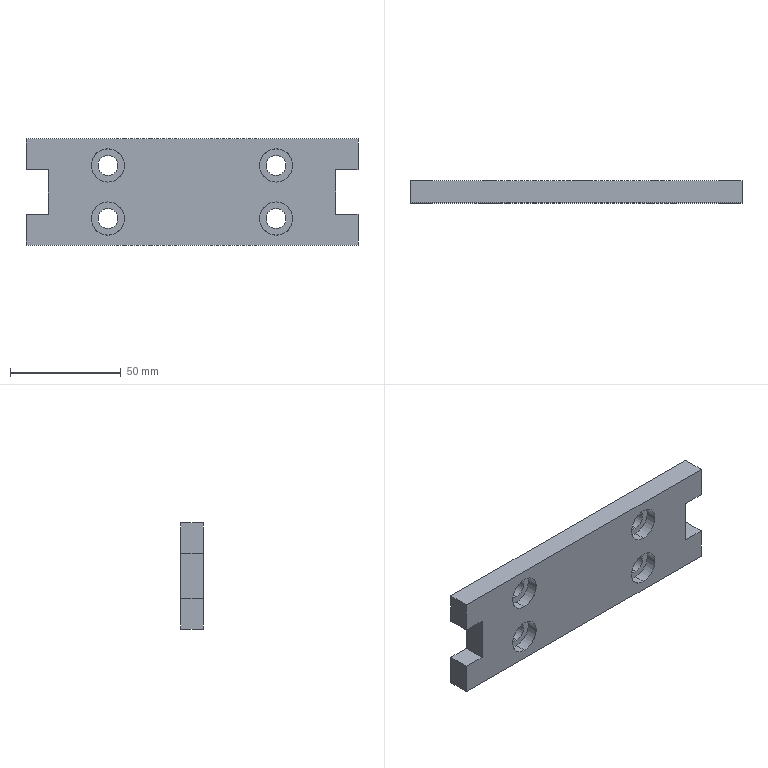Part | SolidWorks | features ICE 2, Extrusion 1, HoleWzd 1 | 1 solid | 45 faces | box 150 x 10 x 48 mm | volume 62310 mm3 | plane 19 | cylinder 18 | cone 8 | commonest cylinder face diameters 15 x10 9 x8
STEP:
#1=CARTESIAN_POINT('',(0.,5.,-7.5));
#2=VERTEX_POINT('',#1);
#3=CARTESIAN_POINT('',(0.,5.,7.5));
#4=VERTEX_POINT('',#3);
#5=CARTESIAN_POINT('',(0.,5.,0.));
#6=DIRECTION('',(0.,1.,0.));
#7=DIRECTION('',(0.,0.,1.));
#8=AXIS2_PLACEMENT_3D('',#5,#6,#7);
#9=CIRCLE('',#8,7.5);
#10=EDGE_CURVE('',#2,#4,#9,.T.);
#11=ORIENTED_EDGE('',*,*,#10,.F.);
#12=CARTESIAN_POINT('',(0.,10.,-7.5));
#13=VERTEX_POINT('',#12);
#14=CARTESIAN_POINT('',(0.,5.,-7.5));
#15=DIRECTION('',(0.,1.,0.));
#16=VECTOR('',#15,1000.);
#17=LINE('',#14,#16);
#18=EDGE_CURVE('',#2,#13,#17,.T.);
#19=ORIENTED_EDGE('',*,*,#18,.T.);
#20=CARTESIAN_POINT('',(0.,10.,7.5));
#21=VERTEX_POINT('',#20);
#22=CARTESIAN_POINT('',(0.,10.,0.));
#23=DIRECTION('',(0.,1.,0.));
#24=DIRECTION('',(0.,0.,1.));
#25=AXIS2_PLACEMENT_3D('',#22,#23,#24);
#26=CIRCLE('',#25,7.5);
#27=EDGE_CURVE('',#13,#21,#26,.T.);
#28=ORIENTED_EDGE('',*,*,#27,.T.);
#29=CARTESIAN_POINT('',(0.,5.,7.5));
#30=DIRECTION('',(0.,1.,0.));
#31=VECTOR('',#30,1000.);
#32=LINE('',#29,#31);
#33=EDGE_CURVE('',#4,#21,#32,.T.);
#34=ORIENTED_EDGE('',*,*,#33,.F.);
#35=EDGE_LOOP('',(#11,#19,#28,#34));
#36=FACE_OUTER_BOUND('',#35,.T.);
#37=CARTESIAN_POINT('',(0.,5.,0.));
#38=DIRECTION('',(0.,1.,0.));
#39=DIRECTION('',(0.,0.,1.));
#40=AXIS2_PLACEMENT_3D('',#37,#38,#39);
#41=CYLINDRICAL_SURFACE('',#40,7.5);
#42=ADVANCED_FACE('',(#36),#41,.F.);
#43=CARTESIAN_POINT('',(38.,0.025,19.5));
#44=VERTEX_POINT('',#43);
#45=CARTESIAN_POINT('',(38.,0.025,4.5));
#46=VERTEX_POINT('',#45);
#47=CARTESIAN_POINT('',(38.,0.025,12.));
#48=DIRECTION('',(0.,-1.,0.));
#49=DIRECTION('',(0.,0.,-1.));
#50=AXIS2_PLACEMENT_3D('',#47,#48,#49);
#51=CIRCLE('',#50,7.5);
#52=EDGE_CURVE('',#44,#46,#51,.T.);
#53=ORIENTED_EDGE('',*,*,#52,.F.);
#54=CARTESIAN_POINT('',(38.,0.,19.525));
#55=VERTEX_POINT('',#54);
#56=CARTESIAN_POINT('',(38.,0.,19.525));
#57=DIRECTION('',(0.,-0.7071,0.7071));
#58=VECTOR('',#57,1000.);
#59=LINE('',#56,#58);
#60=EDGE_CURVE('',#44,#55,#59,.T.);
#61=ORIENTED_EDGE('',*,*,#60,.T.);
#62=CARTESIAN_POINT('',(38.,0.,4.475));
#63=VERTEX_POINT('',#62);
#64=CARTESIAN_POINT('',(38.,0.,12.));
#65=DIRECTION('',(0.,-1.,0.));
#66=DIRECTION('',(0.,0.,-1.));
#67=AXIS2_PLACEMENT_3D('',#64,#65,#66);
#68=CIRCLE('',#67,7.525);
#69=EDGE_CURVE('',#55,#63,#68,.T.);
#70=ORIENTED_EDGE('',*,*,#69,.T.);
#71=CARTESIAN_POINT('',(38.,0.,4.475));
#72=DIRECTION('',(0.,-0.7071,-0.7071));
#73=VECTOR('',#72,1000.);
#74=LINE('',#71,#73);
#75=EDGE_CURVE('',#46,#63,#74,.T.);
#76=ORIENTED_EDGE('',*,*,#75,.F.);
#77=EDGE_LOOP('',(#53,#61,#70,#76));
#78=FACE_OUTER_BOUND('',#77,.T.);
#79=CARTESIAN_POINT('',(38.,0.,12.));
#80=DIRECTION('',(0.,-1.,0.));
#81=DIRECTION('',(0.,0.,-1.));
#82=AXIS2_PLACEMENT_3D('',#79,#80,#81);
#83=CONICAL_SURFACE('',#82,7.525,0.7854);
#84=ADVANCED_FACE('',(#78),#83,.F.);
#85=CARTESIAN_POINT('',(38.,5.,19.5));
#86=VERTEX_POINT('',#85);
#87=CARTESIAN_POINT('',(38.,5.,4.5));
#88=VERTEX_POINT('',#87);
#89=CARTESIAN_POINT('',(38.,5.,12.));
#90=DIRECTION('',(0.,-1.,0.));
#91=DIRECTION('',(0.,0.,-1.));
#92=AXIS2_PLACEMENT_3D('',#89,#90,#91);
#93=CIRCLE('',#92,7.5);
#94=EDGE_CURVE('',#86,#88,#93,.T.);
#95=ORIENTED_EDGE('',*,*,#94,.F.);
#96=CARTESIAN_POINT('',(38.,0.,19.5));
#97=DIRECTION('',(0.,-1.,0.));
#98=VECTOR('',#97,1000.);
#99=LINE('',#96,#98);
#100=EDGE_CURVE('',#86,#44,#99,.T.);
#101=ORIENTED_EDGE('',*,*,#100,.T.);
#102=ORIENTED_EDGE('',*,*,#52,.T.);
#103=CARTESIAN_POINT('',(38.,0.,4.5));
#104=DIRECTION('',(0.,-1.,0.));
#105=VECTOR('',#104,1000.);
#106=LINE('',#103,#105);
#107=EDGE_CURVE('',#88,#46,#106,.T.);
#108=ORIENTED_EDGE('',*,*,#107,.F.);
#109=EDGE_LOOP('',(#95,#101,#102,#108));
#110=FACE_OUTER_BOUND('',#109,.T.);
#111=CARTESIAN_POINT('',(38.,0.,12.));
#112=DIRECTION('',(0.,-1.,0.));
#113=DIRECTION('',(0.,0.,-1.));
#114=AXIS2_PLACEMENT_3D('',#111,#112,#113);
#115=CYLINDRICAL_SURFACE('',#114,7.5);
#116=ADVANCED_FACE('',(#110),#115,.F.);
#117=CARTESIAN_POINT('',(38.,10.,16.5));
#118=VERTEX_POINT('',#117);
#119=CARTESIAN_POINT('',(38.,10.,7.5));
#120=VERTEX_POINT('',#119);
#121=CARTESIAN_POINT('',(38.,10.,12.));
#122=DIRECTION('',(0.,-1.,0.));
#123=DIRECTION('',(0.,0.,-1.));
#124=AXIS2_PLACEMENT_3D('',#121,#122,#123);
#125=CIRCLE('',#124,4.5);
#126=EDGE_CURVE('',#118,#120,#125,.T.);
#127=ORIENTED_EDGE('',*,*,#126,.F.);
#128=CARTESIAN_POINT('',(38.,5.,16.5));
#129=VERTEX_POINT('',#128);
#130=CARTESIAN_POINT('',(38.,0.,16.5));
#131=DIRECTION('',(0.,-1.,0.));
#132=VECTOR('',#131,1000.);
#133=LINE('',#130,#132);
#134=EDGE_CURVE('',#118,#129,#133,.T.);
#135=ORIENTED_EDGE('',*,*,#134,.T.);
#136=CARTESIAN_POINT('',(38.,5.,7.5));
#137=VERTEX_POINT('',#136);
#138=CARTESIAN_POINT('',(38.,5.,12.));
#139=DIRECTION('',(0.,-1.,0.));
#140=DIRECTION('',(0.,0.,-1.));
#141=AXIS2_PLACEMENT_3D('',#138,#139,#140);
#142=CIRCLE('',#141,4.5);
#143=EDGE_CURVE('',#129,#137,#142,.T.);
#144=ORIENTED_EDGE('',*,*,#143,.T.);
#145=CARTESIAN_POINT('',(38.,0.,7.5));
#146=DIRECTION('',(0.,-1.,0.));
#147=VECTOR('',#146,1000.);
#148=LINE('',#145,#147);
#149=EDGE_CURVE('',#120,#137,#148,.T.);
#150=ORIENTED_EDGE('',*,*,#149,.F.);
#151=EDGE_LOOP('',(#127,#135,#144,#150));
#152=FACE_OUTER_BOUND('',#151,.T.);
#153=CARTESIAN_POINT('',(38.,0.,12.));
#154=DIRECTION('',(0.,-1.,0.));
#155=DIRECTION('',(0.,0.,-1.));
#156=AXIS2_PLACEMENT_3D('',#153,#154,#155);
#157=CYLINDRICAL_SURFACE('',#156,4.5);
#158=ADVANCED_FACE('',(#152),#157,.F.);
#159=CARTESIAN_POINT('',(-38.,0.025,19.5));
#160=VERTEX_POINT('',#159);
#161=CARTESIAN_POINT('',(-38.,0.025,4.5));
#162=VERTEX_POINT('',#161);
#163=CARTESIAN_POINT('',(-38.,0.025,12.));
#164=DIRECTION('',(0.,-1.,0.));
#165=DIRECTION('',(0.,0.,-1.));
#166=AXIS2_PLACEMENT_3D('',#163,#164,#165);
#167=CIRCLE('',#166,7.5);
#168=EDGE_CURVE('',#160,#162,#167,.T.);
#169=ORIENTED_EDGE('',*,*,#168,.F.);
#170=CARTESIAN_POINT('',(-38.,0.,19.525));
#171=VERTEX_POINT('',#170);
#172=CARTESIAN_POINT('',(-38.,0.,19.525));
#173=DIRECTION('',(0.,-0.7071,0.7071));
#174=VECTOR('',#173,1000.);
#175=LINE('',#172,#174);
#176=EDGE_CURVE('',#160,#171,#175,.T.);
#177=ORIENTED_EDGE('',*,*,#176,.T.);
#178=CARTESIAN_POINT('',(-38.,0.,4.475));
#179=VERTEX_POINT('',#178);
#180=CARTESIAN_POINT('',(-38.,0.,12.));
#181=DIRECTION('',(0.,-1.,0.));
#182=DIRECTION('',(0.,0.,-1.));
#183=AXIS2_PLACEMENT_3D('',#180,#181,#182);
#184=CIRCLE('',#183,7.525);
#185=EDGE_CURVE('',#171,#179,#184,.T.);
#186=ORIENTED_EDGE('',*,*,#185,.T.);
#187=CARTESIAN_POINT('',(-38.,0.,4.475));
#188=DIRECTION('',(0.,-0.7071,-0.7071));
#189=VECTOR('',#188,1000.);
#190=LINE('',#187,#189);
#191=EDGE_CURVE('',#162,#179,#190,.T.);
#192=ORIENTED_EDGE('',*,*,#191,.F.);
#193=EDGE_LOOP('',(#169,#177,#186,#192));
#194=FACE_OUTER_BOUND('',#193,.T.);
#195=CARTESIAN_POINT('',(-38.,0.,12.));
#196=DIRECTION('',(0.,-1.,0.));
#197=DIRECTION('',(0.,0.,-1.));
#198=AXIS2_PLACEMENT_3D('',#195,#196,#197);
#199=CONICAL_SURFACE('',#198,7.525,0.7854);
#200=ADVANCED_FACE('',(#194),#199,.F.);
#201=CARTESIAN_POINT('',(-38.,5.,19.5));
#202=VERTEX_POINT('',#201);
#203=CARTESIAN_POINT('',(-38.,5.,4.5));
#204=VERTEX_POINT('',#203);
#205=CARTESIAN_POINT('',(-38.,5.,12.));
#206=DIRECTION('',(0.,-1.,0.));
#207=DIRECTION('',(0.,0.,-1.));
#208=AXIS2_PLACEMENT_3D('',#205,#206,#207);
#209=CIRCLE('',#208,7.5);
#210=EDGE_CURVE('',#202,#204,#209,.T.);
#211=ORIENTED_EDGE('',*,*,#210,.F.);
#212=CARTESIAN_POINT('',(-38.,0.,19.5));
#213=DIRECTION('',(0.,-1.,0.));
#214=VECTOR('',#213,1000.);
#215=LINE('',#212,#214);
#216=EDGE_CURVE('',#202,#160,#215,.T.);
#217=ORIENTED_EDGE('',*,*,#216,.T.);
#218=ORIENTED_EDGE('',*,*,#168,.T.);
#219=CARTESIAN_POINT('',(-38.,0.,4.5));
#220=DIRECTION('',(0.,-1.,0.));
#221=VECTOR('',#220,1000.);
#222=LINE('',#219,#221);
#223=EDGE_CURVE('',#204,#162,#222,.T.);
#224=ORIENTED_EDGE('',*,*,#223,.F.);
#225=EDGE_LOOP('',(#211,#217,#218,#224));
#226=FACE_OUTER_BOUND('',#225,.T.);
#227=CARTESIAN_POINT('',(-38.,0.,12.));
#228=DIRECTION('',(0.,-1.,0.));
#229=DIRECTION('',(0.,0.,-1.));
#230=AXIS2_PLACEMENT_3D('',#227,#228,#229);
#231=CYLINDRICAL_SURFACE('',#230,7.5);
#232=ADVANCED_FACE('',(#226),#231,.F.);
#233=CARTESIAN_POINT('',(-38.,10.,16.5));
#234=VERTEX_POINT('',#233);
#235=CARTESIAN_POINT('',(-38.,10.,7.5));
#236=VERTEX_POINT('',#235);
#237=CARTESIAN_POINT('',(-38.,10.,12.));
#238=DIRECTION('',(0.,-1.,0.));
#239=DIRECTION('',(0.,0.,-1.));
#240=AXIS2_PLACEMENT_3D('',#237,#238,#239);
#241=CIRCLE('',#240,4.5);
#242=EDGE_CURVE('',#234,#236,#241,.T.);
#243=ORIENTED_EDGE('',*,*,#242,.F.);
#244=CARTESIAN_POINT('',(-38.,5.,16.5));
#245=VERTEX_POINT('',#244);
#246=CARTESIAN_POINT('',(-38.,0.,16.5));
#247=DIRECTION('',(0.,-1.,0.));
#248=VECTOR('',#247,1000.);
#249=LINE('',#246,#248);
#250=EDGE_CURVE('',#234,#245,#249,.T.);
#251=ORIENTED_EDGE('',*,*,#250,.T.);
#252=CARTESIAN_POINT('',(-38.,5.,7.5));
#253=VERTEX_POINT('',#252);
#254=CARTESIAN_POINT('',(-38.,5.,12.));
#255=DIRECTION('',(0.,-1.,0.));
#256=DIRECTION('',(0.,0.,-1.));
#257=AXIS2_PLACEMENT_3D('',#254,#255,#256);
#258=CIRCLE('',#257,4.5);
#259=EDGE_CURVE('',#245,#253,#258,.T.);
#260=ORIENTED_EDGE('',*,*,#259,.T.);
#261=CARTESIAN_POINT('',(-38.,0.,7.5));
#262=DIRECTION('',(0.,-1.,0.));
#263=VECTOR('',#262,1000.);
#264=LINE('',#261,#263);
#265=EDGE_CURVE('',#236,#253,#264,.T.);
#266=ORIENTED_EDGE('',*,*,#265,.F.);
#267=EDGE_LOOP('',(#243,#251,#260,#266));
#268=FACE_OUTER_BOUND('',#267,.T.);
#269=CARTESIAN_POINT('',(-38.,0.,12.));
#270=DIRECTION('',(0.,-1.,0.));
#271=DIRECTION('',(0.,0.,-1.));
#272=AXIS2_PLACEMENT_3D('',#269,#270,#271);
#273=CYLINDRICAL_SURFACE('',#272,4.5);
#274=ADVANCED_FACE('',(#268),#273,.F.);
#275=CARTESIAN_POINT('',(38.,0.025,-4.5));
#276=VERTEX_POINT('',#275);
#277=CARTESIAN_POINT('',(38.,0.025,-19.5));
#278=VERTEX_POINT('',#277);
#279=CARTESIAN_POINT('',(38.,0.025,-12.));
#280=DIRECTION('',(0.,-1.,0.));
#281=DIRECTION('',(0.,0.,-1.));
#282=AXIS2_PLACEMENT_3D('',#279,#280,#281);
#283=CIRCLE('',#282,7.5);
#284=EDGE_CURVE('',#276,#278,#283,.T.);
#285=ORIENTED_EDGE('',*,*,#284,.F.);
#286=CARTESIAN_POINT('',(38.,0.,-4.475));
#287=VERTEX_POINT('',#286);
#288=CARTESIAN_POINT('',(38.,0.,-4.475));
#289=DIRECTION('',(0.,-0.7071,0.7071));
#290=VECTOR('',#289,1000.);
#291=LINE('',#288,#290);
#292=EDGE_CURVE('',#276,#287,#291,.T.);
#293=ORIENTED_EDGE('',*,*,#292,.T.);
#294=CARTESIAN_POINT('',(38.,0.,-19.525));
#295=VERTEX_POINT('',#294);
#296=CARTESIAN_POINT('',(38.,0.,-12.));
#297=DIRECTION('',(0.,-1.,0.));
#298=DIRECTION('',(0.,0.,-1.));
#299=AXIS2_PLACEMENT_3D('',#296,#297,#298);
#300=CIRCLE('',#299,7.525);
#301=EDGE_CURVE('',#287,#295,#300,.T.);
#302=ORIENTED_EDGE('',*,*,#301,.T.);
#303=CARTESIAN_POINT('',(38.,0.,-19.525));
#304=DIRECTION('',(0.,-0.7071,-0.7071));
#305=VECTOR('',#304,1000.);
#306=LINE('',#303,#305);
#307=EDGE_CURVE('',#278,#295,#306,.T.);
#308=ORIENTED_EDGE('',*,*,#307,.F.);
#309=EDGE_LOOP('',(#285,#293,#302,#308));
#310=FACE_OUTER_BOUND('',#309,.T.);
#311=CARTESIAN_POINT('',(38.,0.,-12.));
#312=DIRECTION('',(0.,-1.,0.));
#313=DIRECTION('',(0.,0.,-1.));
#314=AXIS2_PLACEMENT_3D('',#311,#312,#313);
#315=CONICAL_SURFACE('',#314,7.525,0.7854);
#316=ADVANCED_FACE('',(#310),#315,.F.);
#317=CARTESIAN_POINT('',(38.,5.,-4.5));
#318=VERTEX_POINT('',#317);
#319=CARTESIAN_POINT('',(38.,5.,-19.5));
#320=VERTEX_POINT('',#319);
#321=CARTESIAN_POINT('',(38.,5.,-12.));
#322=DIRECTION('',(0.,-1.,0.));
#323=DIRECTION('',(0.,0.,-1.));
#324=AXIS2_PLACEMENT_3D('',#321,#322,#323);
#325=CIRCLE('',#324,7.5);
#326=EDGE_CURVE('',#318,#320,#325,.T.);
#327=ORIENTED_EDGE('',*,*,#326,.F.);
#328=CARTESIAN_POINT('',(38.,0.,-4.5));
#329=DIRECTION('',(0.,-1.,0.));
#330=VECTOR('',#329,1000.);
#331=LINE('',#328,#330);
#332=EDGE_CURVE('',#318,#276,#331,.T.);
#333=ORIENTED_EDGE('',*,*,#332,.T.);
#334=ORIENTED_EDGE('',*,*,#284,.T.);
#335=CARTESIAN_POINT('',(38.,0.,-19.5));
#336=DIRECTION('',(0.,-1.,0.));
#337=VECTOR('',#336,1000.);
#338=LINE('',#335,#337);
#339=EDGE_CURVE('',#320,#278,#338,.T.);
#340=ORIENTED_EDGE('',*,*,#339,.F.);
#341=EDGE_LOOP('',(#327,#333,#334,#340));
#342=FACE_OUTER_BOUND('',#341,.T.);
#343=CARTESIAN_POINT('',(38.,0.,-12.));
#344=DIRECTION('',(0.,-1.,0.));
#345=DIRECTION('',(0.,0.,-1.));
#346=AXIS2_PLACEMENT_3D('',#343,#344,#345);
#347=CYLINDRICAL_SURFACE('',#346,7.5);
#348=ADVANCED_FACE('',(#342),#347,.F.);
#349=CARTESIAN_POINT('',(38.,10.,-7.5));
#350=VERTEX_POINT('',#349);
#351=CARTESIAN_POINT('',(38.,10.,-16.5));
#352=VERTEX_POINT('',#351);
#353=CARTESIAN_POINT('',(38.,10.,-12.));
#354=DIRECTION('',(0.,-1.,0.));
#355=DIRECTION('',(0.,0.,-1.));
#356=AXIS2_PLACEMENT_3D('',#353,#354,#355);
#357=CIRCLE('',#356,4.5);
#358=EDGE_CURVE('',#350,#352,#357,.T.);
#359=ORIENTED_EDGE('',*,*,#358,.F.);
#360=CARTESIAN_POINT('',(38.,5.,-7.5));
#361=VERTEX_POINT('',#360);
#362=CARTESIAN_POINT('',(38.,0.,-7.5));
#363=DIRECTION('',(0.,-1.,0.));
#364=VECTOR('',#363,1000.);
#365=LINE('',#362,#364);
#366=EDGE_CURVE('',#350,#361,#365,.T.);
#367=ORIENTED_EDGE('',*,*,#366,.T.);
#368=CARTESIAN_POINT('',(38.,5.,-16.5));
#369=VERTEX_POINT('',#368);
#370=CARTESIAN_POINT('',(38.,5.,-12.));
#371=DIRECTION('',(0.,-1.,0.));
#372=DIRECTION('',(0.,0.,-1.));
#373=AXIS2_PLACEMENT_3D('',#370,#371,#372);
#374=CIRCLE('',#373,4.5);
#375=EDGE_CURVE('',#361,#369,#374,.T.);
#376=ORIENTED_EDGE('',*,*,#375,.T.);
#377=CARTESIAN_POINT('',(38.,0.,-16.5));
#378=DIRECTION('',(0.,-1.,0.));
#379=VECTOR('',#378,1000.);
#380=LINE('',#377,#379);
#381=EDGE_CURVE('',#352,#369,#380,.T.);
#382=ORIENTED_EDGE('',*,*,#381,.F.);
#383=EDGE_LOOP('',(#359,#367,#376,#382));
#384=FACE_OUTER_BOUND('',#383,.T.);
#385=CARTESIAN_POINT('',(38.,0.,-12.));
#386=DIRECTION('',(0.,-1.,0.));
#387=DIRECTION('',(0.,0.,-1.));
#388=AXIS2_PLACEMENT_3D('',#385,#386,#387);
#389=CYLINDRICAL_SURFACE('',#388,4.5);
#390=ADVANCED_FACE('',(#384),#389,.F.);
#391=CARTESIAN_POINT('',(-38.,0.025,-4.5));
#392=VERTEX_POINT('',#391);
#393=CARTESIAN_POINT('',(-38.,0.025,-19.5));
#394=VERTEX_POINT('',#393);
#395=CARTESIAN_POINT('',(-38.,0.025,-12.));
#396=DIRECTION('',(0.,-1.,0.));
#397=DIRECTION('',(0.,0.,-1.));
#398=AXIS2_PLACEMENT_3D('',#395,#396,#397);
#399=CIRCLE('',#398,7.5);
#400=EDGE_CURVE('',#392,#394,#399,.T.);
#401=ORIENTED_EDGE('',*,*,#400,.F.);
#402=CARTESIAN_POINT('',(-38.,0.,-4.475));
#403=VERTEX_POINT('',#402);
#404=CARTESIAN_POINT('',(-38.,0.,-4.475));
#405=DIRECTION('',(0.,-0.7071,0.7071));
#406=VECTOR('',#405,1000.);
#407=LINE('',#404,#406);
#408=EDGE_CURVE('',#392,#403,#407,.T.);
#409=ORIENTED_EDGE('',*,*,#408,.T.);
#410=CARTESIAN_POINT('',(-38.,0.,-19.525));
#411=VERTEX_POINT('',#410);
#412=CARTESIAN_POINT('',(-38.,0.,-12.));
#413=DIRECTION('',(0.,-1.,0.));
#414=DIRECTION('',(0.,0.,-1.));
#415=AXIS2_PLACEMENT_3D('',#412,#413,#414);
#416=CIRCLE('',#415,7.525);
#417=EDGE_CURVE('',#403,#411,#416,.T.);
#418=ORIENTED_EDGE('',*,*,#417,.T.);
#419=CARTESIAN_POINT('',(-38.,0.,-19.525));
#420=DIRECTION('',(0.,-0.7071,-0.7071));
#421=VECTOR('',#420,1000.);
#422=LINE('',#419,#421);
#423=EDGE_CURVE('',#394,#411,#422,.T.);
#424=ORIENTED_EDGE('',*,*,#423,.F.);
#425=EDGE_LOOP('',(#401,#409,#418,#424));
#426=FACE_OUTER_BOUND('',#425,.T.);
#427=CARTESIAN_POINT('',(-38.,0.,-12.));
#428=DIRECTION('',(0.,-1.,0.));
#429=DIRECTION('',(0.,0.,-1.));
#430=AXIS2_PLACEMENT_3D('',#427,#428,#429);
#431=CONICAL_SURFACE('',#430,7.525,0.7854);
#432=ADVANCED_FACE('',(#426),#431,.F.);
#433=CARTESIAN_POINT('',(-38.,5.,-4.5));
#434=VERTEX_POINT('',#433);
#435=CARTESIAN_POINT('',(-38.,5.,-19.5));
#436=VERTEX_POINT('',#435);
#437=CARTESIAN_POINT('',(-38.,5.,-12.));
#438=DIRECTION('',(0.,-1.,0.));
#439=DIRECTION('',(0.,0.,-1.));
#440=AXIS2_PLACEMENT_3D('',#437,#438,#439);
#441=CIRCLE('',#440,7.5);
#442=EDGE_CURVE('',#434,#436,#441,.T.);
#443=ORIENTED_EDGE('',*,*,#442,.F.);
#444=CARTESIAN_POINT('',(-38.,0.,-4.5));
#445=DIRECTION('',(0.,-1.,0.));
#446=VECTOR('',#445,1000.);
#447=LINE('',#444,#446);
#448=EDGE_CURVE('',#434,#392,#447,.T.);
#449=ORIENTED_EDGE('',*,*,#448,.T.);
#450=ORIENTED_EDGE('',*,*,#400,.T.);
#451=CARTESIAN_POINT('',(-38.,0.,-19.5));
#452=DIRECTION('',(0.,-1.,0.));
#453=VECTOR('',#452,1000.);
#454=LINE('',#451,#453);
#455=EDGE_CURVE('',#436,#394,#454,.T.);
#456=ORIENTED_EDGE('',*,*,#455,.F.);
#457=EDGE_LOOP('',(#443,#449,#450,#456));
#458=FACE_OUTER_BOUND('',#457,.T.);
#459=CARTESIAN_POINT('',(-38.,0.,-12.));
#460=DIRECTION('',(0.,-1.,0.));
#461=DIRECTION('',(0.,0.,-1.));
#462=AXIS2_PLACEMENT_3D('',#459,#460,#461);
#463=CYLINDRICAL_SURFACE('',#462,7.5);
#464=ADVANCED_FACE('',(#458),#463,.F.);
#465=CARTESIAN_POINT('',(-38.,10.,-7.5));
#466=VERTEX_POINT('',#465);
#467=CARTESIAN_POINT('',(-38.,10.,-16.5));
#468=VERTEX_POINT('',#467);
#469=CARTESIAN_POINT('',(-38.,10.,-12.));
#470=DIRECTION('',(0.,-1.,0.));
#471=DIRECTION('',(0.,0.,-1.));
#472=AXIS2_PLACEMENT_3D('',#469,#470,#471);
#473=CIRCLE('',#472,4.5);
#474=EDGE_CURVE('',#466,#468,#473,.T.);
#475=ORIENTED_EDGE('',*,*,#474,.F.);
#476=CARTESIAN_POINT('',(-38.,5.,-7.5));
#477=VERTEX_POINT('',#476);
#478=CARTESIAN_POINT('',(-38.,0.,-7.5));
#479=DIRECTION('',(0.,-1.,0.));
#480=VECTOR('',#479,1000.);
#481=LINE('',#478,#480);
#482=EDGE_CURVE('',#466,#477,#481,.T.);
#483=ORIENTED_EDGE('',*,*,#482,.T.);
#484=CARTESIAN_POINT('',(-38.,5.,-16.5));
#485=VERTEX_POINT('',#484);
#486=CARTESIAN_POINT('',(-38.,5.,-12.));
#487=DIRECTION('',(0.,-1.,0.));
#488=DIRECTION('',(0.,0.,-1.));
#489=AXIS2_PLACEMENT_3D('',#486,#487,#488);
#490=CIRCLE('',#489,4.5);
#491=EDGE_CURVE('',#477,#485,#490,.T.);
#492=ORIENTED_EDGE('',*,*,#491,.T.);
#493=CARTESIAN_POINT('',(-38.,0.,-16.5));
#494=DIRECTION('',(0.,-1.,0.));
#495=VECTOR('',#494,1000.);
#496=LINE('',#493,#495);
#497=EDGE_CURVE('',#468,#485,#496,.T.);
#498=ORIENTED_EDGE('',*,*,#497,.F.);
#499=EDGE_LOOP('',(#475,#483,#492,#498));
#500=FACE_OUTER_BOUND('',#499,.T.);
#501=CARTESIAN_POINT('',(-38.,0.,-12.));
#502=DIRECTION('',(0.,-1.,0.));
#503=DIRECTION('',(0.,0.,-1.));
#504=AXIS2_PLACEMENT_3D('',#501,#502,#503);
#505=CYLINDRICAL_SURFACE('',#504,4.5);
#506=ADVANCED_FACE('',(#500),#505,.F.);
#507=CARTESIAN_POINT('',(75.,0.,24.));
#508=VERTEX_POINT('',#507);
#509=CARTESIAN_POINT('',(75.,0.,10.));
#510=VERTEX_POINT('',#509);
#511=CARTESIAN_POINT('',(75.,0.,-24.));
#512=DIRECTION('',(0.,0.,-1.));
#513=VECTOR('',#512,1000.);
#514=LINE('',#511,#513);
#515=EDGE_CURVE('',#508,#510,#514,.T.);
#516=ORIENTED_EDGE('',*,*,#515,.T.);
#517=CARTESIAN_POINT('',(75.,10.,10.));
#518=VERTEX_POINT('',#517);
#519=CARTESIAN_POINT('',(75.,10.,10.));
#520=DIRECTION('',(0.,1.,0.));
#521=VECTOR('',#520,1000.);
#522=LINE('',#519,#521);
#523=EDGE_CURVE('',#510,#518,#522,.T.);
#524=ORIENTED_EDGE('',*,*,#523,.T.);
#525=CARTESIAN_POINT('',(75.,10.,24.));
#526=VERTEX_POINT('',#525);
#527=CARTESIAN_POINT('',(75.,10.,-24.));
#528=DIRECTION('',(0.,0.,-1.));
#529=VECTOR('',#528,1000.);
#530=LINE('',#527,#529);
#531=EDGE_CURVE('',#526,#518,#530,.T.);
#532=ORIENTED_EDGE('',*,*,#531,.F.);
#533=CARTESIAN_POINT('',(75.,10.,24.));
#534=DIRECTION('',(0.,-1.,0.));
#535=VECTOR('',#534,1000.);
#536=LINE('',#533,#535);
#537=EDGE_CURVE('',#526,#508,#536,.T.);
#538=ORIENTED_EDGE('',*,*,#537,.T.);
#539=EDGE_LOOP('',(#516,#524,#532,#538));
#540=FACE_OUTER_BOUND('',#539,.T.);
#541=CARTESIAN_POINT('',(75.,10.,-24.));
#542=DIRECTION('',(-1.,0.,0.));
#543=DIRECTION('',(0.,0.,1.));
#544=AXIS2_PLACEMENT_3D('',#541,#542,#543);
#545=PLANE('',#544);
#546=ADVANCED_FACE('',(#540),#545,.F.);
#547=CARTESIAN_POINT('',(-75.,10.,10.));
#548=VERTEX_POINT('',#547);
#549=CARTESIAN_POINT('',(-75.,10.,24.));
#550=VERTEX_POINT('',#549);
#551=CARTESIAN_POINT('',(-75.,10.,-24.));
#552=DIRECTION('',(0.,0.,1.));
#553=VECTOR('',#552,1000.);
#554=LINE('',#551,#553);
#555=EDGE_CURVE('',#548,#550,#554,.T.);
#556=ORIENTED_EDGE('',*,*,#555,.F.);
#557=CARTESIAN_POINT('',(-75.,0.,10.));
#558=VERTEX_POINT('',#557);
#559=CARTESIAN_POINT('',(-75.,10.,10.));
#560=DIRECTION('',(0.,-1.,0.));
#561=VECTOR('',#560,1000.);
#562=LINE('',#559,#561);
#563=EDGE_CURVE('',#548,#558,#562,.T.);
#564=ORIENTED_EDGE('',*,*,#563,.T.);
#565=CARTESIAN_POINT('',(-75.,0.,24.));
#566=VERTEX_POINT('',#565);
#567=CARTESIAN_POINT('',(-75.,0.,-24.));
#568=DIRECTION('',(0.,0.,1.));
#569=VECTOR('',#568,1000.);
#570=LINE('',#567,#569);
#571=EDGE_CURVE('',#558,#566,#570,.T.);
#572=ORIENTED_EDGE('',*,*,#571,.T.);
#573=CARTESIAN_POINT('',(-75.,10.,24.));
#574=DIRECTION('',(0.,-1.,0.));
#575=VECTOR('',#574,1000.);
#576=LINE('',#573,#575);
#577=EDGE_CURVE('',#550,#566,#576,.T.);
#578=ORIENTED_EDGE('',*,*,#577,.F.);
#579=EDGE_LOOP('',(#556,#564,#572,#578));
#580=FACE_OUTER_BOUND('',#579,.T.);
#581=CARTESIAN_POINT('',(-75.,10.,-24.));
#582=DIRECTION('',(1.,0.,0.));
#583=DIRECTION('',(0.,0.,-1.));
#584=AXIS2_PLACEMENT_3D('',#581,#582,#583);
#585=PLANE('',#584);
#586=ADVANCED_FACE('',(#580),#585,.F.);
#587=CARTESIAN_POINT('',(75.,10.,-10.));
#588=VERTEX_POINT('',#587);
#589=CARTESIAN_POINT('',(75.,10.,-24.));
#590=VERTEX_POINT('',#589);
#591=CARTESIAN_POINT('',(75.,10.,-24.));
#592=DIRECTION('',(0.,0.,-1.));
#593=VECTOR('',#592,1000.);
#594=LINE('',#591,#593);
#595=EDGE_CURVE('',#588,#590,#594,.T.);
#596=ORIENTED_EDGE('',*,*,#595,.F.);
#597=CARTESIAN_POINT('',(75.,0.,-10.));
#598=VERTEX_POINT('',#597);
#599=CARTESIAN_POINT('',(75.,10.,-10.));
#600=DIRECTION('',(0.,-1.,0.));
#601=VECTOR('',#600,1000.);
#602=LINE('',#599,#601);
#603=EDGE_CURVE('',#588,#598,#602,.T.);
#604=ORIENTED_EDGE('',*,*,#603,.T.);
#605=CARTESIAN_POINT('',(75.,0.,-24.));
#606=VERTEX_POINT('',#605);
#607=CARTESIAN_POINT('',(75.,0.,-24.));
#608=DIRECTION('',(0.,0.,-1.));
#609=VECTOR('',#608,1000.);
#610=LINE('',#607,#609);
#611=EDGE_CURVE('',#598,#606,#610,.T.);
#612=ORIENTED_EDGE('',*,*,#611,.T.);
#613=CARTESIAN_POINT('',(75.,10.,-24.));
#614=DIRECTION('',(0.,-1.,0.));
#615=VECTOR('',#614,1000.);
#616=LINE('',#613,#615);
#617=EDGE_CURVE('',#590,#606,#616,.T.);
#618=ORIENTED_EDGE('',*,*,#617,.F.);
#619=EDGE_LOOP('',(#596,#604,#612,#618));
#620=FACE_OUTER_BOUND('',#619,.T.);
#621=CARTESIAN_POINT('',(75.,10.,-24.));
#622=DIRECTION('',(-1.,0.,0.));
#623=DIRECTION('',(0.,0.,1.));
#624=AXIS2_PLACEMENT_3D('',#621,#622,#623);
#625=PLANE('',#624);
#626=ADVANCED_FACE('',(#620),#625,.F.);
#627=CARTESIAN_POINT('',(-75.,0.,-24.));
#628=VERTEX_POINT('',#627);
#629=CARTESIAN_POINT('',(-75.,0.,-24.));
#630=DIRECTION('',(-1.,0.,0.));
#631=VECTOR('',#630,1000.);
#632=LINE('',#629,#631);
#633=EDGE_CURVE('',#606,#628,#632,.T.);
#634=ORIENTED_EDGE('',*,*,#633,.T.);
#635=CARTESIAN_POINT('',(-75.,10.,-24.));
#636=VERTEX_POINT('',#635);
#637=CARTESIAN_POINT('',(-75.,10.,-24.));
#638=DIRECTION('',(0.,-1.,0.));
#639=VECTOR('',#638,1000.);
#640=LINE('',#637,#639);
#641=EDGE_CURVE('',#636,#628,#640,.T.);
#642=ORIENTED_EDGE('',*,*,#641,.F.);
#643=CARTESIAN_POINT('',(-75.,10.,-24.));
#644=DIRECTION('',(-1.,0.,0.));
#645=VECTOR('',#644,1000.);
#646=LINE('',#643,#645);
#647=EDGE_CURVE('',#590,#636,#646,.T.);
#648=ORIENTED_EDGE('',*,*,#647,.F.);
#649=ORIENTED_EDGE('',*,*,#617,.T.);
#650=EDGE_LOOP('',(#634,#642,#648,#649));
#651=FACE_OUTER_BOUND('',#650,.T.);
#652=CARTESIAN_POINT('',(-75.,10.,-24.));
#653=DIRECTION('',(0.,0.,1.));
#654=DIRECTION('',(1.,0.,0.));
#655=AXIS2_PLACEMENT_3D('',#652,#653,#654);
#656=PLANE('',#655);
#657=ADVANCED_FACE('',(#651),#656,.F.);
#658=CARTESIAN_POINT('',(-75.,0.,-10.));
#659=VERTEX_POINT('',#658);
#660=CARTESIAN_POINT('',(-75.,0.,-24.));
#661=DIRECTION('',(0.,0.,1.));
#662=VECTOR('',#661,1000.);
#663=LINE('',#660,#662);
#664=EDGE_CURVE('',#628,#659,#663,.T.);
#665=ORIENTED_EDGE('',*,*,#664,.T.);
#666=CARTESIAN_POINT('',(-75.,10.,-10.));
#667=VERTEX_POINT('',#666);
#668=CARTESIAN_POINT('',(-75.,10.,-10.));
#669=DIRECTION('',(0.,1.,0.));
#670=VECTOR('',#669,1000.);
#671=LINE('',#668,#670);
#672=EDGE_CURVE('',#659,#667,#671,.T.);
#673=ORIENTED_EDGE('',*,*,#672,.T.);
#674=CARTESIAN_POINT('',(-75.,10.,-24.));
#675=DIRECTION('',(0.,0.,1.));
#676=VECTOR('',#675,1000.);
#677=LINE('',#674,#676);
#678=EDGE_CURVE('',#636,#667,#677,.T.);
#679=ORIENTED_EDGE('',*,*,#678,.F.);
#680=ORIENTED_EDGE('',*,*,#641,.T.);
#681=EDGE_LOOP('',(#665,#673,#679,#680));
#682=FACE_OUTER_BOUND('',#681,.T.);
#683=CARTESIAN_POINT('',(-75.,10.,-24.));
#684=DIRECTION('',(1.,0.,0.));
#685=DIRECTION('',(0.,0.,-1.));
#686=AXIS2_PLACEMENT_3D('',#683,#684,#685);
#687=PLANE('',#686);
#688=ADVANCED_FACE('',(#682),#687,.F.);
#689=CARTESIAN_POINT('',(-75.,0.,24.));
#690=DIRECTION('',(1.,0.,0.));
#691=VECTOR('',#690,1000.);
#692=LINE('',#689,#691);
#693=EDGE_CURVE('',#566,#508,#692,.T.);
#694=ORIENTED_EDGE('',*,*,#693,.T.);
#695=ORIENTED_EDGE('',*,*,#537,.F.);
#696=CARTESIAN_POINT('',(-75.,10.,24.));
#697=DIRECTION('',(1.,0.,0.));
#698=VECTOR('',#697,1000.);
#699=LINE('',#696,#698);
#700=EDGE_CURVE('',#550,#526,#699,.T.);
#701=ORIENTED_EDGE('',*,*,#700,.F.);
#702=ORIENTED_EDGE('',*,*,#577,.T.);
#703=EDGE_LOOP('',(#694,#695,#701,#702));
#704=FACE_OUTER_BOUND('',#703,.T.);
#705=CARTESIAN_POINT('',(-75.,10.,24.));
#706=DIRECTION('',(0.,0.,-1.));
#707=DIRECTION('',(-1.,0.,0.));
#708=AXIS2_PLACEMENT_3D('',#705,#706,#707);
#709=PLANE('',#708);
#710=ADVANCED_FACE('',(#704),#709,.F.);
#711=CARTESIAN_POINT('',(65.,10.,10.));
#712=VERTEX_POINT('',#711);
#713=CARTESIAN_POINT('',(65.,10.,10.));
#714=DIRECTION('',(1.,0.,0.));
#715=VECTOR('',#714,1000.);
#716=LINE('',#713,#715);
#717=EDGE_CURVE('',#712,#518,#716,.T.);
#718=ORIENTED_EDGE('',*,*,#717,.F.);
#719=CARTESIAN_POINT('',(65.,10.,-10.));
#720=VERTEX_POINT('',#719);
#721=CARTESIAN_POINT('',(65.,10.,10.));
#722=DIRECTION('',(0.,0.,1.));
#723=VECTOR('',#722,1000.);
#724=LINE('',#721,#723);
#725=EDGE_CURVE('',#720,#712,#724,.T.);
#726=ORIENTED_EDGE('',*,*,#725,.F.);
#727=CARTESIAN_POINT('',(65.,10.,-10.));
#728=DIRECTION('',(-1.,0.,0.));
#729=VECTOR('',#728,1000.);
#730=LINE('',#727,#729);
#731=EDGE_CURVE('',#588,#720,#730,.T.);
#732=ORIENTED_EDGE('',*,*,#731,.F.);
#733=ORIENTED_EDGE('',*,*,#595,.T.);
#734=ORIENTED_EDGE('',*,*,#647,.T.);
#735=ORIENTED_EDGE('',*,*,#678,.T.);
#736=CARTESIAN_POINT('',(-65.,10.,-10.));
#737=VERTEX_POINT('',#736);
#738=CARTESIAN_POINT('',(-65.,10.,-10.));
#739=DIRECTION('',(-1.,0.,0.));
#740=VECTOR('',#739,1000.);
#741=LINE('',#738,#740);
#742=EDGE_CURVE('',#737,#667,#741,.T.);
#743=ORIENTED_EDGE('',*,*,#742,.F.);
#744=CARTESIAN_POINT('',(-65.,10.,10.));
#745=VERTEX_POINT('',#744);
#746=CARTESIAN_POINT('',(-65.,10.,10.));
#747=DIRECTION('',(0.,0.,-1.));
#748=VECTOR('',#747,1000.);
#749=LINE('',#746,#748);
#750=EDGE_CURVE('',#745,#737,#749,.T.);
#751=ORIENTED_EDGE('',*,*,#750,.F.);
#752=CARTESIAN_POINT('',(-65.,10.,10.));
#753=DIRECTION('',(1.,0.,0.));
#754=VECTOR('',#753,1000.);
#755=LINE('',#752,#754);
#756=EDGE_CURVE('',#548,#745,#755,.T.);
#757=ORIENTED_EDGE('',*,*,#756,.F.);
#758=ORIENTED_EDGE('',*,*,#555,.T.);
#759=ORIENTED_EDGE('',*,*,#700,.T.);
#760=ORIENTED_EDGE('',*,*,#531,.T.);
#761=EDGE_LOOP('',(#718,#726,#732,#733,#734,#735,#743,#751,#757,#758,#759,#760));
#762=FACE_OUTER_BOUND('',#761,.T.);
#763=CARTESIAN_POINT('',(0.,10.,0.));
#764=DIRECTION('',(0.,1.,0.));
#765=DIRECTION('',(0.,0.,1.));
#766=AXIS2_PLACEMENT_3D('',#763,#764,#765);
#767=CIRCLE('',#766,7.5);
#768=EDGE_CURVE('',#21,#13,#767,.T.);
#769=ORIENTED_EDGE('',*,*,#768,.F.);
#770=ORIENTED_EDGE('',*,*,#27,.F.);
#771=EDGE_LOOP('',(#769,#770));
#772=FACE_BOUND('',#771,.T.);
#773=CARTESIAN_POINT('',(38.,10.,12.));
#774=DIRECTION('',(0.,-1.,0.));
#775=DIRECTION('',(0.,0.,-1.));
#776=AXIS2_PLACEMENT_3D('',#773,#774,#775);
#777=CIRCLE('',#776,4.5);
#778=EDGE_CURVE('',#120,#118,#777,.T.);
#779=ORIENTED_EDGE('',*,*,#778,.T.);
#780=ORIENTED_EDGE('',*,*,#126,.T.);
#781=EDGE_LOOP('',(#779,#780));
#782=FACE_BOUND('',#781,.T.);
#783=CARTESIAN_POINT('',(-38.,10.,12.));
#784=DIRECTION('',(0.,-1.,0.));
#785=DIRECTION('',(0.,0.,-1.));
#786=AXIS2_PLACEMENT_3D('',#783,#784,#785);
#787=CIRCLE('',#786,4.5);
#788=EDGE_CURVE('',#236,#234,#787,.T.);
#789=ORIENTED_EDGE('',*,*,#788,.T.);
#790=ORIENTED_EDGE('',*,*,#242,.T.);
#791=EDGE_LOOP('',(#789,#790));
#792=FACE_BOUND('',#791,.T.);
#793=CARTESIAN_POINT('',(38.,10.,-12.));
#794=DIRECTION('',(0.,-1.,0.));
#795=DIRECTION('',(0.,0.,-1.));
#796=AXIS2_PLACEMENT_3D('',#793,#794,#795);
#797=CIRCLE('',#796,4.5);
#798=EDGE_CURVE('',#352,#350,#797,.T.);
#799=ORIENTED_EDGE('',*,*,#798,.T.);
#800=ORIENTED_EDGE('',*,*,#358,.T.);
#801=EDGE_LOOP('',(#799,#800));
#802=FACE_BOUND('',#801,.T.);
#803=CARTESIAN_POINT('',(-38.,10.,-12.));
#804=DIRECTION('',(0.,-1.,0.));
#805=DIRECTION('',(0.,0.,-1.));
#806=AXIS2_PLACEMENT_3D('',#803,#804,#805);
#807=CIRCLE('',#806,4.5);
#808=EDGE_CURVE('',#468,#466,#807,.T.);
#809=ORIENTED_EDGE('',*,*,#808,.T.);
#810=ORIENTED_EDGE('',*,*,#474,.T.);
#811=EDGE_LOOP('',(#809,#810));
#812=FACE_BOUND('',#811,.T.);
#813=CARTESIAN_POINT('',(0.,10.,0.));
#814=DIRECTION('',(0.,1.,0.));
#815=DIRECTION('',(0.,0.,1.));
#816=AXIS2_PLACEMENT_3D('',#813,#814,#815);
#817=PLANE('',#816);
#818=ADVANCED_FACE('',(#762,#772,#782,#792,#802,#812),#817,.T.);
#819=CARTESIAN_POINT('',(38.,0.,12.));
#820=DIRECTION('',(0.,-1.,0.));
#821=DIRECTION('',(0.,0.,-1.));
#822=AXIS2_PLACEMENT_3D('',#819,#820,#821);
#823=CIRCLE('',#822,7.525);
#824=EDGE_CURVE('',#63,#55,#823,.T.);
#825=ORIENTED_EDGE('',*,*,#824,.F.);
#826=ORIENTED_EDGE('',*,*,#69,.F.);
#827=EDGE_LOOP('',(#825,#826));
#828=FACE_BOUND('',#827,.T.);
#829=CARTESIAN_POINT('',(-38.,0.,12.));
#830=DIRECTION('',(0.,-1.,0.));
#831=DIRECTION('',(0.,0.,-1.));
#832=AXIS2_PLACEMENT_3D('',#829,#830,#831);
#833=CIRCLE('',#832,7.525);
#834=EDGE_CURVE('',#179,#171,#833,.T.);
#835=ORIENTED_EDGE('',*,*,#834,.F.);
#836=ORIENTED_EDGE('',*,*,#185,.F.);
#837=EDGE_LOOP('',(#835,#836));
#838=FACE_BOUND('',#837,.T.);
#839=CARTESIAN_POINT('',(38.,0.,-12.));
#840=DIRECTION('',(0.,-1.,0.));
#841=DIRECTION('',(0.,0.,-1.));
#842=AXIS2_PLACEMENT_3D('',#839,#840,#841);
#843=CIRCLE('',#842,7.525);
#844=EDGE_CURVE('',#295,#287,#843,.T.);
#845=ORIENTED_EDGE('',*,*,#844,.F.);
#846=ORIENTED_EDGE('',*,*,#301,.F.);
#847=EDGE_LOOP('',(#845,#846));
#848=FACE_BOUND('',#847,.T.);
#849=CARTESIAN_POINT('',(-38.,0.,-12.));
#850=DIRECTION('',(0.,-1.,0.));
#851=DIRECTION('',(0.,0.,-1.));
#852=AXIS2_PLACEMENT_3D('',#849,#850,#851);
#853=CIRCLE('',#852,7.525);
#854=EDGE_CURVE('',#411,#403,#853,.T.);
#855=ORIENTED_EDGE('',*,*,#854,.F.);
#856=ORIENTED_EDGE('',*,*,#417,.F.);
#857=EDGE_LOOP('',(#855,#856));
#858=FACE_BOUND('',#857,.T.);
#859=CARTESIAN_POINT('',(65.,0.,-10.));
#860=VERTEX_POINT('',#859);
#861=CARTESIAN_POINT('',(65.,0.,10.));
#862=VERTEX_POINT('',#861);
#863=CARTESIAN_POINT('',(65.,0.,10.));
#864=DIRECTION('',(0.,0.,1.));
#865=VECTOR('',#864,1000.);
#866=LINE('',#863,#865);
#867=EDGE_CURVE('',#860,#862,#866,.T.);
#868=ORIENTED_EDGE('',*,*,#867,.T.);
#869=CARTESIAN_POINT('',(65.,0.,10.));
#870=DIRECTION('',(1.,0.,0.));
#871=VECTOR('',#870,1000.);
#872=LINE('',#869,#871);
#873=EDGE_CURVE('',#862,#510,#872,.T.);
#874=ORIENTED_EDGE('',*,*,#873,.T.);
#875=ORIENTED_EDGE('',*,*,#515,.F.);
#876=ORIENTED_EDGE('',*,*,#693,.F.);
#877=ORIENTED_EDGE('',*,*,#571,.F.);
#878=CARTESIAN_POINT('',(-65.,0.,10.));
#879=VERTEX_POINT('',#878);
#880=CARTESIAN_POINT('',(0.,0.,10.));
#881=DIRECTION('',(1.,0.,0.));
#882=VECTOR('',#881,1000.);
#883=LINE('',#880,#882);
#884=EDGE_CURVE('',#558,#879,#883,.T.);
#885=ORIENTED_EDGE('',*,*,#884,.T.);
#886=CARTESIAN_POINT('',(-65.,0.,-10.));
#887=VERTEX_POINT('',#886);
#888=CARTESIAN_POINT('',(-65.,0.,10.));
#889=DIRECTION('',(0.,0.,-1.));
#890=VECTOR('',#889,1000.);
#891=LINE('',#888,#890);
#892=EDGE_CURVE('',#879,#887,#891,.T.);
#893=ORIENTED_EDGE('',*,*,#892,.T.);
#894=CARTESIAN_POINT('',(-65.,0.,-10.));
#895=DIRECTION('',(-1.,0.,0.));
#896=VECTOR('',#895,1000.);
#897=LINE('',#894,#896);
#898=EDGE_CURVE('',#887,#659,#897,.T.);
#899=ORIENTED_EDGE('',*,*,#898,.T.);
#900=ORIENTED_EDGE('',*,*,#664,.F.);
#901=ORIENTED_EDGE('',*,*,#633,.F.);
#902=ORIENTED_EDGE('',*,*,#611,.F.);
#903=CARTESIAN_POINT('',(0.,0.,-10.));
#904=DIRECTION('',(-1.,0.,0.));
#905=VECTOR('',#904,1000.);
#906=LINE('',#903,#905);
#907=EDGE_CURVE('',#598,#860,#906,.T.);
#908=ORIENTED_EDGE('',*,*,#907,.T.);
#909=EDGE_LOOP('',(#868,#874,#875,#876,#877,#885,#893,#899,#900,#901,#902,#908));
#910=FACE_OUTER_BOUND('',#909,.T.);
#911=CARTESIAN_POINT('',(0.,0.,0.));
#912=DIRECTION('',(0.,1.,0.));
#913=DIRECTION('',(0.,0.,1.));
#914=AXIS2_PLACEMENT_3D('',#911,#912,#913);
#915=PLANE('',#914);
#916=ADVANCED_FACE('',(#828,#838,#848,#858,#910),#915,.F.);
#917=ORIENTED_EDGE('',*,*,#482,.F.);
#918=ORIENTED_EDGE('',*,*,#808,.F.);
#919=ORIENTED_EDGE('',*,*,#497,.T.);
#920=CARTESIAN_POINT('',(-38.,5.,-12.));
#921=DIRECTION('',(0.,-1.,0.));
#922=DIRECTION('',(0.,0.,-1.));
#923=AXIS2_PLACEMENT_3D('',#920,#921,#922);
#924=CIRCLE('',#923,4.5);
#925=EDGE_CURVE('',#485,#477,#924,.T.);
#926=ORIENTED_EDGE('',*,*,#925,.T.);
#927=EDGE_LOOP('',(#917,#918,#919,#926));
#928=FACE_OUTER_BOUND('',#927,.T.);
#929=CARTESIAN_POINT('',(-38.,0.,-12.));
#930=DIRECTION('',(0.,-1.,0.));
#931=DIRECTION('',(0.,0.,-1.));
#932=AXIS2_PLACEMENT_3D('',#929,#930,#931);
#933=CYLINDRICAL_SURFACE('',#932,4.5);
#934=ADVANCED_FACE('',(#928),#933,.F.);
#935=ORIENTED_EDGE('',*,*,#925,.F.);
#936=ORIENTED_EDGE('',*,*,#491,.F.);
#937=EDGE_LOOP('',(#935,#936));
#938=FACE_BOUND('',#937,.T.);
#939=CARTESIAN_POINT('',(-38.,5.,-12.));
#940=DIRECTION('',(0.,-1.,0.));
#941=DIRECTION('',(0.,0.,-1.));
#942=AXIS2_PLACEMENT_3D('',#939,#940,#941);
#943=CIRCLE('',#942,7.5);
#944=EDGE_CURVE('',#436,#434,#943,.T.);
#945=ORIENTED_EDGE('',*,*,#944,.T.);
#946=ORIENTED_EDGE('',*,*,#442,.T.);
#947=EDGE_LOOP('',(#945,#946));
#948=FACE_OUTER_BOUND('',#947,.T.);
#949=CARTESIAN_POINT('',(-33.5,5.,-12.));
#950=DIRECTION('',(0.,1.,0.));
#951=DIRECTION('',(0.,0.,1.));
#952=AXIS2_PLACEMENT_3D('',#949,#950,#951);
#953=PLANE('',#952);
#954=ADVANCED_FACE('',(#938,#948),#953,.F.);
#955=ORIENTED_EDGE('',*,*,#448,.F.);
#956=ORIENTED_EDGE('',*,*,#944,.F.);
#957=ORIENTED_EDGE('',*,*,#455,.T.);
#958=CARTESIAN_POINT('',(-38.,0.025,-12.));
#959=DIRECTION('',(0.,-1.,0.));
#960=DIRECTION('',(0.,0.,-1.));
#961=AXIS2_PLACEMENT_3D('',#958,#959,#960);
#962=CIRCLE('',#961,7.5);
#963=EDGE_CURVE('',#394,#392,#962,.T.);
#964=ORIENTED_EDGE('',*,*,#963,.T.);
#965=EDGE_LOOP('',(#955,#956,#957,#964));
#966=FACE_OUTER_BOUND('',#965,.T.);
#967=CARTESIAN_POINT('',(-38.,0.,-12.));
#968=DIRECTION('',(0.,-1.,0.));
#969=DIRECTION('',(0.,0.,-1.));
#970=AXIS2_PLACEMENT_3D('',#967,#968,#969);
#971=CYLINDRICAL_SURFACE('',#970,7.5);
#972=ADVANCED_FACE('',(#966),#971,.F.);
#973=ORIENTED_EDGE('',*,*,#408,.F.);
#974=ORIENTED_EDGE('',*,*,#963,.F.);
#975=ORIENTED_EDGE('',*,*,#423,.T.);
#976=ORIENTED_EDGE('',*,*,#854,.T.);
#977=EDGE_LOOP('',(#973,#974,#975,#976));
#978=FACE_OUTER_BOUND('',#977,.T.);
#979=CARTESIAN_POINT('',(-38.,0.,-12.));
#980=DIRECTION('',(0.,-1.,0.));
#981=DIRECTION('',(0.,0.,-1.));
#982=AXIS2_PLACEMENT_3D('',#979,#980,#981);
#983=CONICAL_SURFACE('',#982,7.525,0.7854);
#984=ADVANCED_FACE('',(#978),#983,.F.);
#985=ORIENTED_EDGE('',*,*,#366,.F.);
#986=ORIENTED_EDGE('',*,*,#798,.F.);
#987=ORIENTED_EDGE('',*,*,#381,.T.);
#988=CARTESIAN_POINT('',(38.,5.,-12.));
#989=DIRECTION('',(0.,-1.,0.));
#990=DIRECTION('',(0.,0.,-1.));
#991=AXIS2_PLACEMENT_3D('',#988,#989,#990);
#992=CIRCLE('',#991,4.5);
#993=EDGE_CURVE('',#369,#361,#992,.T.);
#994=ORIENTED_EDGE('',*,*,#993,.T.);
#995=EDGE_LOOP('',(#985,#986,#987,#994));
#996=FACE_OUTER_BOUND('',#995,.T.);
#997=CARTESIAN_POINT('',(38.,0.,-12.));
#998=DIRECTION('',(0.,-1.,0.));
#999=DIRECTION('',(0.,0.,-1.));
#1000=AXIS2_PLACEMENT_3D('',#997,#998,#999);
#1001=CYLINDRICAL_SURFACE('',#1000,4.5);
#1002=ADVANCED_FACE('',(#996),#1001,.F.);
#1003=ORIENTED_EDGE('',*,*,#993,.F.);
#1004=ORIENTED_EDGE('',*,*,#375,.F.);
#1005=EDGE_LOOP('',(#1003,#1004));
#1006=FACE_BOUND('',#1005,.T.);
#1007=CARTESIAN_POINT('',(38.,5.,-12.));
#1008=DIRECTION('',(0.,-1.,0.));
#1009=DIRECTION('',(0.,0.,-1.));
#1010=AXIS2_PLACEMENT_3D('',#1007,#1008,#1009);
#1011=CIRCLE('',#1010,7.5);
#1012=EDGE_CURVE('',#320,#318,#1011,.T.);
#1013=ORIENTED_EDGE('',*,*,#1012,.T.);
#1014=ORIENTED_EDGE('',*,*,#326,.T.);
#1015=EDGE_LOOP('',(#1013,#1014));
#1016=FACE_OUTER_BOUND('',#1015,.T.);
#1017=CARTESIAN_POINT('',(42.5,5.,-12.));
#1018=DIRECTION('',(0.,1.,0.));
#1019=DIRECTION('',(0.,0.,1.));
#1020=AXIS2_PLACEMENT_3D('',#1017,#1018,#1019);
#1021=PLANE('',#1020);
#1022=ADVANCED_FACE('',(#1006,#1016),#1021,.F.);
#1023=ORIENTED_EDGE('',*,*,#332,.F.);
#1024=ORIENTED_EDGE('',*,*,#1012,.F.);
#1025=ORIENTED_EDGE('',*,*,#339,.T.);
#1026=CARTESIAN_POINT('',(38.,0.025,-12.));
#1027=DIRECTION('',(0.,-1.,0.));
#1028=DIRECTION('',(0.,0.,-1.));
#1029=AXIS2_PLACEMENT_3D('',#1026,#1027,#1028);
#1030=CIRCLE('',#1029,7.5);
#1031=EDGE_CURVE('',#278,#276,#1030,.T.);
#1032=ORIENTED_EDGE('',*,*,#1031,.T.);
#1033=EDGE_LOOP('',(#1023,#1024,#1025,#1032));
#1034=FACE_OUTER_BOUND('',#1033,.T.);
#1035=CARTESIAN_POINT('',(38.,0.,-12.));
#1036=DIRECTION('',(0.,-1.,0.));
#1037=DIRECTION('',(0.,0.,-1.));
#1038=AXIS2_PLACEMENT_3D('',#1035,#1036,#1037);
#1039=CYLINDRICAL_SURFACE('',#1038,7.5);
#1040=ADVANCED_FACE('',(#1034),#1039,.F.);
#1041=ORIENTED_EDGE('',*,*,#292,.F.);
#1042=ORIENTED_EDGE('',*,*,#1031,.F.);
#1043=ORIENTED_EDGE('',*,*,#307,.T.);
#1044=ORIENTED_EDGE('',*,*,#844,.T.);
#1045=EDGE_LOOP('',(#1041,#1042,#1043,#1044));
#1046=FACE_OUTER_BOUND('',#1045,.T.);
#1047=CARTESIAN_POINT('',(38.,0.,-12.));
#1048=DIRECTION('',(0.,-1.,0.));
#1049=DIRECTION('',(0.,0.,-1.));
#1050=AXIS2_PLACEMENT_3D('',#1047,#1048,#1049);
#1051=CONICAL_SURFACE('',#1050,7.525,0.7854);
#1052=ADVANCED_FACE('',(#1046),#1051,.F.);
#1053=ORIENTED_EDGE('',*,*,#250,.F.);
#1054=ORIENTED_EDGE('',*,*,#788,.F.);
#1055=ORIENTED_EDGE('',*,*,#265,.T.);
#1056=CARTESIAN_POINT('',(-38.,5.,12.));
#1057=DIRECTION('',(0.,-1.,0.));
#1058=DIRECTION('',(0.,0.,-1.));
#1059=AXIS2_PLACEMENT_3D('',#1056,#1057,#1058);
#1060=CIRCLE('',#1059,4.5);
#1061=EDGE_CURVE('',#253,#245,#1060,.T.);
#1062=ORIENTED_EDGE('',*,*,#1061,.T.);
#1063=EDGE_LOOP('',(#1053,#1054,#1055,#1062));
#1064=FACE_OUTER_BOUND('',#1063,.T.);
#1065=CARTESIAN_POINT('',(-38.,0.,12.));
#1066=DIRECTION('',(0.,-1.,0.));
#1067=DIRECTION('',(0.,0.,-1.));
#1068=AXIS2_PLACEMENT_3D('',#1065,#1066,#1067);
#1069=CYLINDRICAL_SURFACE('',#1068,4.5);
#1070=ADVANCED_FACE('',(#1064),#1069,.F.);
#1071=ORIENTED_EDGE('',*,*,#1061,.F.);
#1072=ORIENTED_EDGE('',*,*,#259,.F.);
#1073=EDGE_LOOP('',(#1071,#1072));
#1074=FACE_BOUND('',#1073,.T.);
#1075=CARTESIAN_POINT('',(-38.,5.,12.));
#1076=DIRECTION('',(0.,-1.,0.));
#1077=DIRECTION('',(0.,0.,-1.));
#1078=AXIS2_PLACEMENT_3D('',#1075,#1076,#1077);
#1079=CIRCLE('',#1078,7.5);
#1080=EDGE_CURVE('',#204,#202,#1079,.T.);
#1081=ORIENTED_EDGE('',*,*,#1080,.T.);
#1082=ORIENTED_EDGE('',*,*,#210,.T.);
#1083=EDGE_LOOP('',(#1081,#1082));
#1084=FACE_OUTER_BOUND('',#1083,.T.);
#1085=CARTESIAN_POINT('',(-33.5,5.,12.));
#1086=DIRECTION('',(0.,1.,0.));
#1087=DIRECTION('',(0.,0.,1.));
#1088=AXIS2_PLACEMENT_3D('',#1085,#1086,#1087);
#1089=PLANE('',#1088);
#1090=ADVANCED_FACE('',(#1074,#1084),#1089,.F.);
#1091=ORIENTED_EDGE('',*,*,#216,.F.);
#1092=ORIENTED_EDGE('',*,*,#1080,.F.);
#1093=ORIENTED_EDGE('',*,*,#223,.T.);
#1094=CARTESIAN_POINT('',(-38.,0.025,12.));
#1095=DIRECTION('',(0.,-1.,0.));
#1096=DIRECTION('',(0.,0.,-1.));
#1097=AXIS2_PLACEMENT_3D('',#1094,#1095,#1096);
#1098=CIRCLE('',#1097,7.5);
#1099=EDGE_CURVE('',#162,#160,#1098,.T.);
#1100=ORIENTED_EDGE('',*,*,#1099,.T.);
#1101=EDGE_LOOP('',(#1091,#1092,#1093,#1100));
#1102=FACE_OUTER_BOUND('',#1101,.T.);
#1103=CARTESIAN_POINT('',(-38.,0.,12.));
#1104=DIRECTION('',(0.,-1.,0.));
#1105=DIRECTION('',(0.,0.,-1.));
#1106=AXIS2_PLACEMENT_3D('',#1103,#1104,#1105);
#1107=CYLINDRICAL_SURFACE('',#1106,7.5);
#1108=ADVANCED_FACE('',(#1102),#1107,.F.);
#1109=ORIENTED_EDGE('',*,*,#176,.F.);
#1110=ORIENTED_EDGE('',*,*,#1099,.F.);
#1111=ORIENTED_EDGE('',*,*,#191,.T.);
#1112=ORIENTED_EDGE('',*,*,#834,.T.);
#1113=EDGE_LOOP('',(#1109,#1110,#1111,#1112));
#1114=FACE_OUTER_BOUND('',#1113,.T.);
#1115=CARTESIAN_POINT('',(-38.,0.,12.));
#1116=DIRECTION('',(0.,-1.,0.));
#1117=DIRECTION('',(0.,0.,-1.));
#1118=AXIS2_PLACEMENT_3D('',#1115,#1116,#1117);
#1119=CONICAL_SURFACE('',#1118,7.525,0.7854);
#1120=ADVANCED_FACE('',(#1114),#1119,.F.);
#1121=ORIENTED_EDGE('',*,*,#134,.F.);
#1122=ORIENTED_EDGE('',*,*,#778,.F.);
#1123=ORIENTED_EDGE('',*,*,#149,.T.);
#1124=CARTESIAN_POINT('',(38.,5.,12.));
#1125=DIRECTION('',(0.,-1.,0.));
#1126=DIRECTION('',(0.,0.,-1.));
#1127=AXIS2_PLACEMENT_3D('',#1124,#1125,#1126);
#1128=CIRCLE('',#1127,4.5);
#1129=EDGE_CURVE('',#137,#129,#1128,.T.);
#1130=ORIENTED_EDGE('',*,*,#1129,.T.);
#1131=EDGE_LOOP('',(#1121,#1122,#1123,#1130));
#1132=FACE_OUTER_BOUND('',#1131,.T.);
#1133=CARTESIAN_POINT('',(38.,0.,12.));
#1134=DIRECTION('',(0.,-1.,0.));
#1135=DIRECTION('',(0.,0.,-1.));
#1136=AXIS2_PLACEMENT_3D('',#1133,#1134,#1135);
#1137=CYLINDRICAL_SURFACE('',#1136,4.5);
#1138=ADVANCED_FACE('',(#1132),#1137,.F.);
#1139=ORIENTED_EDGE('',*,*,#1129,.F.);
#1140=ORIENTED_EDGE('',*,*,#143,.F.);
#1141=EDGE_LOOP('',(#1139,#1140));
#1142=FACE_BOUND('',#1141,.T.);
#1143=CARTESIAN_POINT('',(38.,5.,12.));
#1144=DIRECTION('',(0.,-1.,0.));
#1145=DIRECTION('',(0.,0.,-1.));
#1146=AXIS2_PLACEMENT_3D('',#1143,#1144,#1145);
#1147=CIRCLE('',#1146,7.5);
#1148=EDGE_CURVE('',#88,#86,#1147,.T.);
#1149=ORIENTED_EDGE('',*,*,#1148,.T.);
#1150=ORIENTED_EDGE('',*,*,#94,.T.);
#1151=EDGE_LOOP('',(#1149,#1150));
#1152=FACE_OUTER_BOUND('',#1151,.T.);
#1153=CARTESIAN_POINT('',(42.5,5.,12.));
#1154=DIRECTION('',(0.,1.,0.));
#1155=DIRECTION('',(0.,0.,1.));
#1156=AXIS2_PLACEMENT_3D('',#1153,#1154,#1155);
#1157=PLANE('',#1156);
#1158=ADVANCED_FACE('',(#1142,#1152),#1157,.F.);
#1159=ORIENTED_EDGE('',*,*,#100,.F.);
#1160=ORIENTED_EDGE('',*,*,#1148,.F.);
#1161=ORIENTED_EDGE('',*,*,#107,.T.);
#1162=CARTESIAN_POINT('',(38.,0.025,12.));
#1163=DIRECTION('',(0.,-1.,0.));
#1164=DIRECTION('',(0.,0.,-1.));
#1165=AXIS2_PLACEMENT_3D('',#1162,#1163,#1164);
#1166=CIRCLE('',#1165,7.5);
#1167=EDGE_CURVE('',#46,#44,#1166,.T.);
#1168=ORIENTED_EDGE('',*,*,#1167,.T.);
#1169=EDGE_LOOP('',(#1159,#1160,#1161,#1168));
#1170=FACE_OUTER_BOUND('',#1169,.T.);
#1171=CARTESIAN_POINT('',(38.,0.,12.));
#1172=DIRECTION('',(0.,-1.,0.));
#1173=DIRECTION('',(0.,0.,-1.));
#1174=AXIS2_PLACEMENT_3D('',#1171,#1172,#1173);
#1175=CYLINDRICAL_SURFACE('',#1174,7.5);
#1176=ADVANCED_FACE('',(#1170),#1175,.F.);
#1177=ORIENTED_EDGE('',*,*,#60,.F.);
#1178=ORIENTED_EDGE('',*,*,#1167,.F.);
#1179=ORIENTED_EDGE('',*,*,#75,.T.);
#1180=ORIENTED_EDGE('',*,*,#824,.T.);
#1181=EDGE_LOOP('',(#1177,#1178,#1179,#1180));
#1182=FACE_OUTER_BOUND('',#1181,.T.);
#1183=CARTESIAN_POINT('',(38.,0.,12.));
#1184=DIRECTION('',(0.,-1.,0.));
#1185=DIRECTION('',(0.,0.,-1.));
#1186=AXIS2_PLACEMENT_3D('',#1183,#1184,#1185);
#1187=CONICAL_SURFACE('',#1186,7.525,0.7854);
#1188=ADVANCED_FACE('',(#1182),#1187,.F.);
#1189=ORIENTED_EDGE('',*,*,#18,.F.);
#1190=CARTESIAN_POINT('',(0.,5.,0.));
#1191=DIRECTION('',(0.,1.,0.));
#1192=DIRECTION('',(0.,0.,1.));
#1193=AXIS2_PLACEMENT_3D('',#1190,#1191,#1192);
#1194=CIRCLE('',#1193,7.5);
#1195=EDGE_CURVE('',#4,#2,#1194,.T.);
#1196=ORIENTED_EDGE('',*,*,#1195,.F.);
#1197=ORIENTED_EDGE('',*,*,#33,.T.);
#1198=ORIENTED_EDGE('',*,*,#768,.T.);
#1199=EDGE_LOOP('',(#1189,#1196,#1197,#1198));
#1200=FACE_OUTER_BOUND('',#1199,.T.);
#1201=CARTESIAN_POINT('',(0.,5.,0.));
#1202=DIRECTION('',(0.,1.,0.));
#1203=DIRECTION('',(0.,0.,1.));
#1204=AXIS2_PLACEMENT_3D('',#1201,#1202,#1203);
#1205=CYLINDRICAL_SURFACE('',#1204,7.5);
#1206=ADVANCED_FACE('',(#1200),#1205,.F.);
#1207=ORIENTED_EDGE('',*,*,#1195,.T.);
#1208=ORIENTED_EDGE('',*,*,#10,.T.);
#1209=EDGE_LOOP('',(#1207,#1208));
#1210=FACE_OUTER_BOUND('',#1209,.T.);
#1211=CARTESIAN_POINT('',(0.,5.,0.));
#1212=DIRECTION('',(0.,1.,0.));
#1213=DIRECTION('',(0.,0.,1.));
#1214=AXIS2_PLACEMENT_3D('',#1211,#1212,#1213);
#1215=PLANE('',#1214);
#1216=ADVANCED_FACE('',(#1210),#1215,.T.);
#1217=ORIENTED_EDGE('',*,*,#756,.T.);
#1218=CARTESIAN_POINT('',(-65.,0.,10.));
#1219=DIRECTION('',(0.,1.,0.));
#1220=VECTOR('',#1219,1000.);
#1221=LINE('',#1218,#1220);
#1222=EDGE_CURVE('',#879,#745,#1221,.T.);
#1223=ORIENTED_EDGE('',*,*,#1222,.F.);
#1224=ORIENTED_EDGE('',*,*,#884,.F.);
#1225=ORIENTED_EDGE('',*,*,#563,.F.);
#1226=EDGE_LOOP('',(#1217,#1223,#1224,#1225));
#1227=FACE_OUTER_BOUND('',#1226,.T.);
#1228=CARTESIAN_POINT('',(-65.,0.,10.));
#1229=DIRECTION('',(0.,0.,1.));
#1230=DIRECTION('',(1.,0.,0.));
#1231=AXIS2_PLACEMENT_3D('',#1228,#1229,#1230);
#1232=PLANE('',#1231);
#1233=ADVANCED_FACE('',(#1227),#1232,.F.);
#1234=ORIENTED_EDGE('',*,*,#898,.F.);
#1235=CARTESIAN_POINT('',(-65.,0.,-10.));
#1236=DIRECTION('',(0.,1.,0.));
#1237=VECTOR('',#1236,1000.);
#1238=LINE('',#1235,#1237);
#1239=EDGE_CURVE('',#887,#737,#1238,.T.);
#1240=ORIENTED_EDGE('',*,*,#1239,.T.);
#1241=ORIENTED_EDGE('',*,*,#742,.T.);
#1242=ORIENTED_EDGE('',*,*,#672,.F.);
#1243=EDGE_LOOP('',(#1234,#1240,#1241,#1242));
#1244=FACE_OUTER_BOUND('',#1243,.T.);
#1245=CARTESIAN_POINT('',(-65.,0.,-10.));
#1246=DIRECTION('',(0.,0.,-1.));
#1247=DIRECTION('',(-1.,0.,0.));
#1248=AXIS2_PLACEMENT_3D('',#1245,#1246,#1247);
#1249=PLANE('',#1248);
#1250=ADVANCED_FACE('',(#1244),#1249,.F.);
#1251=ORIENTED_EDGE('',*,*,#750,.T.);
#1252=ORIENTED_EDGE('',*,*,#1239,.F.);
#1253=ORIENTED_EDGE('',*,*,#892,.F.);
#1254=ORIENTED_EDGE('',*,*,#1222,.T.);
#1255=EDGE_LOOP('',(#1251,#1252,#1253,#1254));
#1256=FACE_OUTER_BOUND('',#1255,.T.);
#1257=CARTESIAN_POINT('',(-65.,0.,10.));
#1258=DIRECTION('',(1.,0.,0.));
#1259=DIRECTION('',(0.,0.,-1.));
#1260=AXIS2_PLACEMENT_3D('',#1257,#1258,#1259);
#1261=PLANE('',#1260);
#1262=ADVANCED_FACE('',(#1256),#1261,.F.);
#1263=ORIENTED_EDGE('',*,*,#873,.F.);
#1264=CARTESIAN_POINT('',(65.,0.,10.));
#1265=DIRECTION('',(0.,1.,0.));
#1266=VECTOR('',#1265,1000.);
#1267=LINE('',#1264,#1266);
#1268=EDGE_CURVE('',#862,#712,#1267,.T.);
#1269=ORIENTED_EDGE('',*,*,#1268,.T.);
#1270=ORIENTED_EDGE('',*,*,#717,.T.);
#1271=ORIENTED_EDGE('',*,*,#523,.F.);
#1272=EDGE_LOOP('',(#1263,#1269,#1270,#1271));
#1273=FACE_OUTER_BOUND('',#1272,.T.);
#1274=CARTESIAN_POINT('',(65.,0.,10.));
#1275=DIRECTION('',(0.,0.,1.));
#1276=DIRECTION('',(1.,0.,0.));
#1277=AXIS2_PLACEMENT_3D('',#1274,#1275,#1276);
#1278=PLANE('',#1277);
#1279=ADVANCED_FACE('',(#1273),#1278,.F.);
#1280=ORIENTED_EDGE('',*,*,#731,.T.);
#1281=CARTESIAN_POINT('',(65.,0.,-10.));
#1282=DIRECTION('',(0.,1.,0.));
#1283=VECTOR('',#1282,1000.);
#1284=LINE('',#1281,#1283);
#1285=EDGE_CURVE('',#860,#720,#1284,.T.);
#1286=ORIENTED_EDGE('',*,*,#1285,.F.);
#1287=ORIENTED_EDGE('',*,*,#907,.F.);
#1288=ORIENTED_EDGE('',*,*,#603,.F.);
#1289=EDGE_LOOP('',(#1280,#1286,#1287,#1288));
#1290=FACE_OUTER_BOUND('',#1289,.T.);
#1291=CARTESIAN_POINT('',(65.,0.,-10.));
#1292=DIRECTION('',(0.,0.,-1.));
#1293=DIRECTION('',(-1.,0.,0.));
#1294=AXIS2_PLACEMENT_3D('',#1291,#1292,#1293);
#1295=PLANE('',#1294);
#1296=ADVANCED_FACE('',(#1290),#1295,.F.);
#1297=ORIENTED_EDGE('',*,*,#725,.T.);
#1298=ORIENTED_EDGE('',*,*,#1268,.F.);
#1299=ORIENTED_EDGE('',*,*,#867,.F.);
#1300=ORIENTED_EDGE('',*,*,#1285,.T.);
#1301=EDGE_LOOP('',(#1297,#1298,#1299,#1300));
#1302=FACE_OUTER_BOUND('',#1301,.T.);
#1303=CARTESIAN_POINT('',(65.,0.,10.));
#1304=DIRECTION('',(-1.,0.,0.));
#1305=DIRECTION('',(0.,0.,1.));
#1306=AXIS2_PLACEMENT_3D('',#1303,#1304,#1305);
#1307=PLANE('',#1306);
#1308=ADVANCED_FACE('',(#1302),#1307,.F.);
#1309=CLOSED_SHELL('',(#42,#84,#116,#158,#200,#232,#274,#316,#348,#390,#432,#464,#506,#546,#586,#626,#657,#688,#710,#818,#916,#934,#954,#972,#984,#1002,#1022,#1040,#1052,#1070,#1090,#1108,#1120,#1138,#1158,#1176,#1188,#1206,#1216,#1233,#1250,#1262,#1279,#1296,#1308));
#1310=MANIFOLD_SOLID_BREP('',#1309);
#1311=CARTESIAN_POINT('',(0.,0.,0.));
#1312=DIRECTION('',(0.,0.,1.));
#1313=DIRECTION('',(1.,0.,0.));
#1314=AXIS2_PLACEMENT_3D('',#1311,#1312,#1313);
#1315=(LENGTH_UNIT()NAMED_UNIT(*)SI_UNIT(.MILLI.,.METRE.));
#1316=UNCERTAINTY_MEASURE_WITH_UNIT(LENGTH_MEASURE(0.00001),#1315,'','');
#1317=(NAMED_UNIT(*)PLANE_ANGLE_UNIT()SI_UNIT($,.RADIAN.));
#1318=(NAMED_UNIT(*)SI_UNIT($,.STERADIAN.)SOLID_ANGLE_UNIT());
#1319=(GEOMETRIC_REPRESENTATION_CONTEXT(3)GLOBAL_UNCERTAINTY_ASSIGNED_CONTEXT((#1316))GLOBAL_UNIT_ASSIGNED_CONTEXT((#1315,#1317,#1318))REPRESENTATION_CONTEXT('',''));
#1320=ADVANCED_BREP_SHAPE_REPRESENTATION('',(#1310,#1314),#1319);